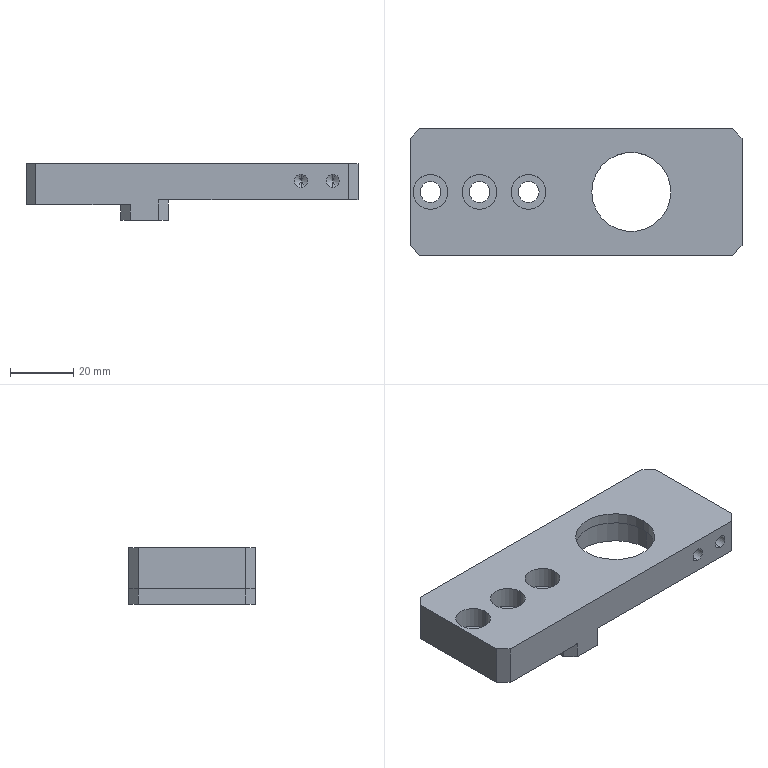Part | SolidWorks | features ICE 5, HoleWzd 2, Chamfer 1, Extrusion 1, MirrorPattern 1 | 1 solid | 57 faces | box 105 x 40 x 18 mm | volume 43487 mm3 | cylinder 26 | plane 23 | cone 8 | commonest cylinder face diameters 4.2 x8 6.6 x6 11 x6 10 x2 25 x2 28 x2